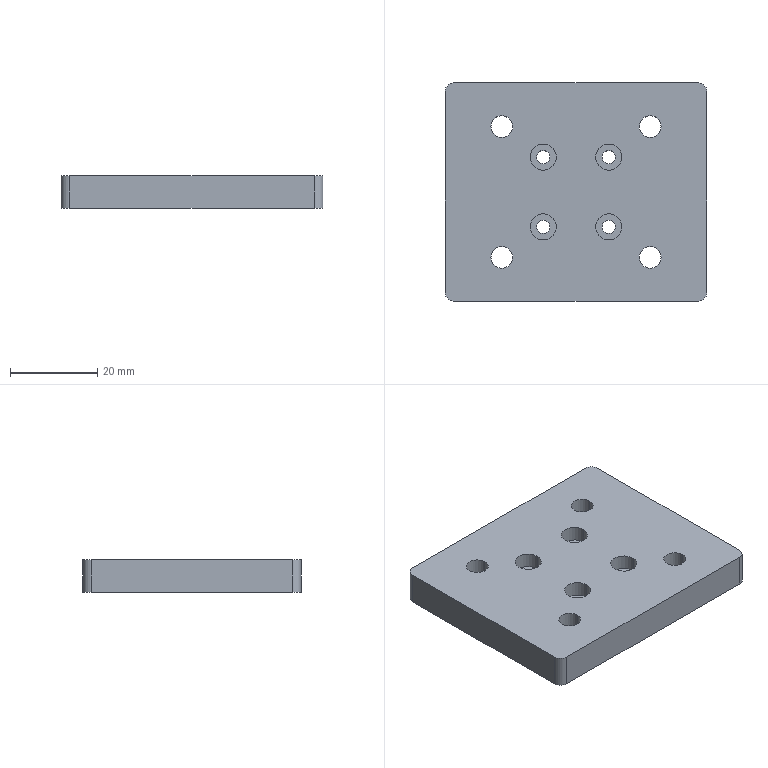Part | SolidWorks | features BaseBody 1 | 1 solid | 38 faces | box 60 x 50 x 7.5 mm | volume 21376 mm3 | cylinder 28 | plane 10 | commonest cylinder face diameters 3 x8 5 x8 6 x8 4 x4
STEP:
#1=CARTESIAN_POINT('',(19.5,-15.,7.5));
#2=VERTEX_POINT('',#1);
#3=CARTESIAN_POINT('',(14.5,-15.,7.5));
#4=VERTEX_POINT('',#3);
#5=CARTESIAN_POINT('',(17.,-15.,7.5));
#6=DIRECTION('',(0.,0.,-1.));
#7=DIRECTION('',(-1.,0.,0.));
#8=AXIS2_PLACEMENT_3D('',#5,#6,#7);
#9=CIRCLE('',#8,2.5);
#10=EDGE_CURVE('',#2,#4,#9,.T.);
#11=ORIENTED_EDGE('',*,*,#10,.F.);
#12=CARTESIAN_POINT('',(19.5,-15.,0.));
#13=VERTEX_POINT('',#12);
#14=CARTESIAN_POINT('',(19.5,-15.,7.5));
#15=DIRECTION('',(0.,0.,-1.));
#16=VECTOR('',#15,1000.);
#17=LINE('',#14,#16);
#18=EDGE_CURVE('',#2,#13,#17,.T.);
#19=ORIENTED_EDGE('',*,*,#18,.T.);
#20=CARTESIAN_POINT('',(14.5,-15.,0.));
#21=VERTEX_POINT('',#20);
#22=CARTESIAN_POINT('',(17.,-15.,0.));
#23=DIRECTION('',(0.,0.,-1.));
#24=DIRECTION('',(-1.,0.,0.));
#25=AXIS2_PLACEMENT_3D('',#22,#23,#24);
#26=CIRCLE('',#25,2.5);
#27=EDGE_CURVE('',#13,#21,#26,.T.);
#28=ORIENTED_EDGE('',*,*,#27,.T.);
#29=CARTESIAN_POINT('',(14.5,-15.,7.5));
#30=DIRECTION('',(0.,0.,-1.));
#31=VECTOR('',#30,1000.);
#32=LINE('',#29,#31);
#33=EDGE_CURVE('',#4,#21,#32,.T.);
#34=ORIENTED_EDGE('',*,*,#33,.F.);
#35=EDGE_LOOP('',(#11,#19,#28,#34));
#36=FACE_OUTER_BOUND('',#35,.T.);
#37=CARTESIAN_POINT('',(17.,-15.,7.5));
#38=DIRECTION('',(0.,0.,-1.));
#39=DIRECTION('',(-1.,0.,0.));
#40=AXIS2_PLACEMENT_3D('',#37,#38,#39);
#41=CYLINDRICAL_SURFACE('',#40,2.5);
#42=ADVANCED_FACE('',(#36),#41,.F.);
#43=CARTESIAN_POINT('',(19.5,15.,7.5));
#44=VERTEX_POINT('',#43);
#45=CARTESIAN_POINT('',(14.5,15.,7.5));
#46=VERTEX_POINT('',#45);
#47=CARTESIAN_POINT('',(17.,15.,7.5));
#48=DIRECTION('',(0.,0.,-1.));
#49=DIRECTION('',(-1.,0.,0.));
#50=AXIS2_PLACEMENT_3D('',#47,#48,#49);
#51=CIRCLE('',#50,2.5);
#52=EDGE_CURVE('',#44,#46,#51,.T.);
#53=ORIENTED_EDGE('',*,*,#52,.F.);
#54=CARTESIAN_POINT('',(19.5,15.,0.));
#55=VERTEX_POINT('',#54);
#56=CARTESIAN_POINT('',(19.5,15.,7.5));
#57=DIRECTION('',(0.,0.,-1.));
#58=VECTOR('',#57,1000.);
#59=LINE('',#56,#58);
#60=EDGE_CURVE('',#44,#55,#59,.T.);
#61=ORIENTED_EDGE('',*,*,#60,.T.);
#62=CARTESIAN_POINT('',(14.5,15.,0.));
#63=VERTEX_POINT('',#62);
#64=CARTESIAN_POINT('',(17.,15.,0.));
#65=DIRECTION('',(0.,0.,-1.));
#66=DIRECTION('',(-1.,0.,0.));
#67=AXIS2_PLACEMENT_3D('',#64,#65,#66);
#68=CIRCLE('',#67,2.5);
#69=EDGE_CURVE('',#55,#63,#68,.T.);
#70=ORIENTED_EDGE('',*,*,#69,.T.);
#71=CARTESIAN_POINT('',(14.5,15.,7.5));
#72=DIRECTION('',(0.,0.,-1.));
#73=VECTOR('',#72,1000.);
#74=LINE('',#71,#73);
#75=EDGE_CURVE('',#46,#63,#74,.T.);
#76=ORIENTED_EDGE('',*,*,#75,.F.);
#77=EDGE_LOOP('',(#53,#61,#70,#76));
#78=FACE_OUTER_BOUND('',#77,.T.);
#79=CARTESIAN_POINT('',(17.,15.,7.5));
#80=DIRECTION('',(0.,0.,-1.));
#81=DIRECTION('',(-1.,0.,0.));
#82=AXIS2_PLACEMENT_3D('',#79,#80,#81);
#83=CYLINDRICAL_SURFACE('',#82,2.5);
#84=ADVANCED_FACE('',(#78),#83,.F.);
#85=CARTESIAN_POINT('',(-6.,8.,4.));
#86=VERTEX_POINT('',#85);
#87=CARTESIAN_POINT('',(-9.,8.,4.));
#88=VERTEX_POINT('',#87);
#89=CARTESIAN_POINT('',(-7.5,8.,4.));
#90=DIRECTION('',(0.,0.,-1.));
#91=DIRECTION('',(-1.,0.,0.));
#92=AXIS2_PLACEMENT_3D('',#89,#90,#91);
#93=CIRCLE('',#92,1.5);
#94=EDGE_CURVE('',#86,#88,#93,.T.);
#95=ORIENTED_EDGE('',*,*,#94,.F.);
#96=CARTESIAN_POINT('',(-6.,8.,0.));
#97=VERTEX_POINT('',#96);
#98=CARTESIAN_POINT('',(-6.,8.,7.5));
#99=DIRECTION('',(0.,0.,-1.));
#100=VECTOR('',#99,1000.);
#101=LINE('',#98,#100);
#102=EDGE_CURVE('',#86,#97,#101,.T.);
#103=ORIENTED_EDGE('',*,*,#102,.T.);
#104=CARTESIAN_POINT('',(-9.,8.,0.));
#105=VERTEX_POINT('',#104);
#106=CARTESIAN_POINT('',(-7.5,8.,0.));
#107=DIRECTION('',(0.,0.,-1.));
#108=DIRECTION('',(-1.,0.,0.));
#109=AXIS2_PLACEMENT_3D('',#106,#107,#108);
#110=CIRCLE('',#109,1.5);
#111=EDGE_CURVE('',#97,#105,#110,.T.);
#112=ORIENTED_EDGE('',*,*,#111,.T.);
#113=CARTESIAN_POINT('',(-9.,8.,7.5));
#114=DIRECTION('',(0.,0.,-1.));
#115=VECTOR('',#114,1000.);
#116=LINE('',#113,#115);
#117=EDGE_CURVE('',#88,#105,#116,.T.);
#118=ORIENTED_EDGE('',*,*,#117,.F.);
#119=EDGE_LOOP('',(#95,#103,#112,#118));
#120=FACE_OUTER_BOUND('',#119,.T.);
#121=CARTESIAN_POINT('',(-7.5,8.,7.5));
#122=DIRECTION('',(0.,0.,-1.));
#123=DIRECTION('',(-1.,0.,0.));
#124=AXIS2_PLACEMENT_3D('',#121,#122,#123);
#125=CYLINDRICAL_SURFACE('',#124,1.5);
#126=ADVANCED_FACE('',(#120),#125,.F.);
#127=CARTESIAN_POINT('',(9.,8.,4.));
#128=VERTEX_POINT('',#127);
#129=CARTESIAN_POINT('',(6.,8.,4.));
#130=VERTEX_POINT('',#129);
#131=CARTESIAN_POINT('',(7.5,8.,4.));
#132=DIRECTION('',(0.,0.,-1.));
#133=DIRECTION('',(-1.,0.,0.));
#134=AXIS2_PLACEMENT_3D('',#131,#132,#133);
#135=CIRCLE('',#134,1.5);
#136=EDGE_CURVE('',#128,#130,#135,.T.);
#137=ORIENTED_EDGE('',*,*,#136,.F.);
#138=CARTESIAN_POINT('',(9.,8.,0.));
#139=VERTEX_POINT('',#138);
#140=CARTESIAN_POINT('',(9.,8.,7.5));
#141=DIRECTION('',(0.,0.,-1.));
#142=VECTOR('',#141,1000.);
#143=LINE('',#140,#142);
#144=EDGE_CURVE('',#128,#139,#143,.T.);
#145=ORIENTED_EDGE('',*,*,#144,.T.);
#146=CARTESIAN_POINT('',(6.,8.,0.));
#147=VERTEX_POINT('',#146);
#148=CARTESIAN_POINT('',(7.5,8.,0.));
#149=DIRECTION('',(0.,0.,-1.));
#150=DIRECTION('',(-1.,0.,0.));
#151=AXIS2_PLACEMENT_3D('',#148,#149,#150);
#152=CIRCLE('',#151,1.5);
#153=EDGE_CURVE('',#139,#147,#152,.T.);
#154=ORIENTED_EDGE('',*,*,#153,.T.);
#155=CARTESIAN_POINT('',(6.,8.,7.5));
#156=DIRECTION('',(0.,0.,-1.));
#157=VECTOR('',#156,1000.);
#158=LINE('',#155,#157);
#159=EDGE_CURVE('',#130,#147,#158,.T.);
#160=ORIENTED_EDGE('',*,*,#159,.F.);
#161=EDGE_LOOP('',(#137,#145,#154,#160));
#162=FACE_OUTER_BOUND('',#161,.T.);
#163=CARTESIAN_POINT('',(7.5,8.,7.5));
#164=DIRECTION('',(0.,0.,-1.));
#165=DIRECTION('',(-1.,0.,0.));
#166=AXIS2_PLACEMENT_3D('',#163,#164,#165);
#167=CYLINDRICAL_SURFACE('',#166,1.5);
#168=ADVANCED_FACE('',(#162),#167,.F.);
#169=CARTESIAN_POINT('',(9.,-8.,4.));
#170=VERTEX_POINT('',#169);
#171=CARTESIAN_POINT('',(6.,-8.,4.));
#172=VERTEX_POINT('',#171);
#173=CARTESIAN_POINT('',(7.5,-8.,4.));
#174=DIRECTION('',(0.,0.,-1.));
#175=DIRECTION('',(-1.,0.,0.));
#176=AXIS2_PLACEMENT_3D('',#173,#174,#175);
#177=CIRCLE('',#176,1.5);
#178=EDGE_CURVE('',#170,#172,#177,.T.);
#179=ORIENTED_EDGE('',*,*,#178,.F.);
#180=CARTESIAN_POINT('',(9.,-8.,0.));
#181=VERTEX_POINT('',#180);
#182=CARTESIAN_POINT('',(9.,-8.,7.5));
#183=DIRECTION('',(0.,0.,-1.));
#184=VECTOR('',#183,1000.);
#185=LINE('',#182,#184);
#186=EDGE_CURVE('',#170,#181,#185,.T.);
#187=ORIENTED_EDGE('',*,*,#186,.T.);
#188=CARTESIAN_POINT('',(6.,-8.,0.));
#189=VERTEX_POINT('',#188);
#190=CARTESIAN_POINT('',(7.5,-8.,0.));
#191=DIRECTION('',(0.,0.,-1.));
#192=DIRECTION('',(-1.,0.,0.));
#193=AXIS2_PLACEMENT_3D('',#190,#191,#192);
#194=CIRCLE('',#193,1.5);
#195=EDGE_CURVE('',#181,#189,#194,.T.);
#196=ORIENTED_EDGE('',*,*,#195,.T.);
#197=CARTESIAN_POINT('',(6.,-8.,7.5));
#198=DIRECTION('',(0.,0.,-1.));
#199=VECTOR('',#198,1000.);
#200=LINE('',#197,#199);
#201=EDGE_CURVE('',#172,#189,#200,.T.);
#202=ORIENTED_EDGE('',*,*,#201,.F.);
#203=EDGE_LOOP('',(#179,#187,#196,#202));
#204=FACE_OUTER_BOUND('',#203,.T.);
#205=CARTESIAN_POINT('',(7.5,-8.,7.5));
#206=DIRECTION('',(0.,0.,-1.));
#207=DIRECTION('',(-1.,0.,0.));
#208=AXIS2_PLACEMENT_3D('',#205,#206,#207);
#209=CYLINDRICAL_SURFACE('',#208,1.5);
#210=ADVANCED_FACE('',(#204),#209,.F.);
#211=CARTESIAN_POINT('',(-6.,-8.,4.));
#212=VERTEX_POINT('',#211);
#213=CARTESIAN_POINT('',(-9.,-8.,4.));
#214=VERTEX_POINT('',#213);
#215=CARTESIAN_POINT('',(-7.5,-8.,4.));
#216=DIRECTION('',(0.,0.,-1.));
#217=DIRECTION('',(-1.,0.,0.));
#218=AXIS2_PLACEMENT_3D('',#215,#216,#217);
#219=CIRCLE('',#218,1.5);
#220=EDGE_CURVE('',#212,#214,#219,.T.);
#221=ORIENTED_EDGE('',*,*,#220,.F.);
#222=CARTESIAN_POINT('',(-6.,-8.,0.));
#223=VERTEX_POINT('',#222);
#224=CARTESIAN_POINT('',(-6.,-8.,7.5));
#225=DIRECTION('',(0.,0.,-1.));
#226=VECTOR('',#225,1000.);
#227=LINE('',#224,#226);
#228=EDGE_CURVE('',#212,#223,#227,.T.);
#229=ORIENTED_EDGE('',*,*,#228,.T.);
#230=CARTESIAN_POINT('',(-9.,-8.,0.));
#231=VERTEX_POINT('',#230);
#232=CARTESIAN_POINT('',(-7.5,-8.,0.));
#233=DIRECTION('',(0.,0.,-1.));
#234=DIRECTION('',(-1.,0.,0.));
#235=AXIS2_PLACEMENT_3D('',#232,#233,#234);
#236=CIRCLE('',#235,1.5);
#237=EDGE_CURVE('',#223,#231,#236,.T.);
#238=ORIENTED_EDGE('',*,*,#237,.T.);
#239=CARTESIAN_POINT('',(-9.,-8.,7.5));
#240=DIRECTION('',(0.,0.,-1.));
#241=VECTOR('',#240,1000.);
#242=LINE('',#239,#241);
#243=EDGE_CURVE('',#214,#231,#242,.T.);
#244=ORIENTED_EDGE('',*,*,#243,.F.);
#245=EDGE_LOOP('',(#221,#229,#238,#244));
#246=FACE_OUTER_BOUND('',#245,.T.);
#247=CARTESIAN_POINT('',(-7.5,-8.,7.5));
#248=DIRECTION('',(0.,0.,-1.));
#249=DIRECTION('',(-1.,0.,0.));
#250=AXIS2_PLACEMENT_3D('',#247,#248,#249);
#251=CYLINDRICAL_SURFACE('',#250,1.5);
#252=ADVANCED_FACE('',(#246),#251,.F.);
#253=CARTESIAN_POINT('',(-14.5,15.,7.5));
#254=VERTEX_POINT('',#253);
#255=CARTESIAN_POINT('',(-19.5,15.,7.5));
#256=VERTEX_POINT('',#255);
#257=CARTESIAN_POINT('',(-17.,15.,7.5));
#258=DIRECTION('',(0.,0.,-1.));
#259=DIRECTION('',(-1.,0.,0.));
#260=AXIS2_PLACEMENT_3D('',#257,#258,#259);
#261=CIRCLE('',#260,2.5);
#262=EDGE_CURVE('',#254,#256,#261,.T.);
#263=ORIENTED_EDGE('',*,*,#262,.F.);
#264=CARTESIAN_POINT('',(-14.5,15.,0.));
#265=VERTEX_POINT('',#264);
#266=CARTESIAN_POINT('',(-14.5,15.,7.5));
#267=DIRECTION('',(0.,0.,-1.));
#268=VECTOR('',#267,1000.);
#269=LINE('',#266,#268);
#270=EDGE_CURVE('',#254,#265,#269,.T.);
#271=ORIENTED_EDGE('',*,*,#270,.T.);
#272=CARTESIAN_POINT('',(-19.5,15.,0.));
#273=VERTEX_POINT('',#272);
#274=CARTESIAN_POINT('',(-17.,15.,0.));
#275=DIRECTION('',(0.,0.,-1.));
#276=DIRECTION('',(-1.,0.,0.));
#277=AXIS2_PLACEMENT_3D('',#274,#275,#276);
#278=CIRCLE('',#277,2.5);
#279=EDGE_CURVE('',#265,#273,#278,.T.);
#280=ORIENTED_EDGE('',*,*,#279,.T.);
#281=CARTESIAN_POINT('',(-19.5,15.,7.5));
#282=DIRECTION('',(0.,0.,-1.));
#283=VECTOR('',#282,1000.);
#284=LINE('',#281,#283);
#285=EDGE_CURVE('',#256,#273,#284,.T.);
#286=ORIENTED_EDGE('',*,*,#285,.F.);
#287=EDGE_LOOP('',(#263,#271,#280,#286));
#288=FACE_OUTER_BOUND('',#287,.T.);
#289=CARTESIAN_POINT('',(-17.,15.,7.5));
#290=DIRECTION('',(0.,0.,-1.));
#291=DIRECTION('',(-1.,0.,0.));
#292=AXIS2_PLACEMENT_3D('',#289,#290,#291);
#293=CYLINDRICAL_SURFACE('',#292,2.5);
#294=ADVANCED_FACE('',(#288),#293,.F.);
#295=CARTESIAN_POINT('',(-14.5,-15.,7.5));
#296=VERTEX_POINT('',#295);
#297=CARTESIAN_POINT('',(-19.5,-15.,7.5));
#298=VERTEX_POINT('',#297);
#299=CARTESIAN_POINT('',(-17.,-15.,7.5));
#300=DIRECTION('',(0.,0.,-1.));
#301=DIRECTION('',(-1.,0.,0.));
#302=AXIS2_PLACEMENT_3D('',#299,#300,#301);
#303=CIRCLE('',#302,2.5);
#304=EDGE_CURVE('',#296,#298,#303,.T.);
#305=ORIENTED_EDGE('',*,*,#304,.F.);
#306=CARTESIAN_POINT('',(-14.5,-15.,0.));
#307=VERTEX_POINT('',#306);
#308=CARTESIAN_POINT('',(-14.5,-15.,7.5));
#309=DIRECTION('',(0.,0.,-1.));
#310=VECTOR('',#309,1000.);
#311=LINE('',#308,#310);
#312=EDGE_CURVE('',#296,#307,#311,.T.);
#313=ORIENTED_EDGE('',*,*,#312,.T.);
#314=CARTESIAN_POINT('',(-19.5,-15.,0.));
#315=VERTEX_POINT('',#314);
#316=CARTESIAN_POINT('',(-17.,-15.,0.));
#317=DIRECTION('',(0.,0.,-1.));
#318=DIRECTION('',(-1.,0.,0.));
#319=AXIS2_PLACEMENT_3D('',#316,#317,#318);
#320=CIRCLE('',#319,2.5);
#321=EDGE_CURVE('',#307,#315,#320,.T.);
#322=ORIENTED_EDGE('',*,*,#321,.T.);
#323=CARTESIAN_POINT('',(-19.5,-15.,7.5));
#324=DIRECTION('',(0.,0.,-1.));
#325=VECTOR('',#324,1000.);
#326=LINE('',#323,#325);
#327=EDGE_CURVE('',#298,#315,#326,.T.);
#328=ORIENTED_EDGE('',*,*,#327,.F.);
#329=EDGE_LOOP('',(#305,#313,#322,#328));
#330=FACE_OUTER_BOUND('',#329,.T.);
#331=CARTESIAN_POINT('',(-17.,-15.,7.5));
#332=DIRECTION('',(0.,0.,-1.));
#333=DIRECTION('',(-1.,0.,0.));
#334=AXIS2_PLACEMENT_3D('',#331,#332,#333);
#335=CYLINDRICAL_SURFACE('',#334,2.5);
#336=ADVANCED_FACE('',(#330),#335,.F.);
#337=CARTESIAN_POINT('',(-10.5,8.,4.));
#338=VERTEX_POINT('',#337);
#339=CARTESIAN_POINT('',(-4.5,8.,4.));
#340=VERTEX_POINT('',#339);
#341=CARTESIAN_POINT('',(-7.5,8.,4.));
#342=DIRECTION('',(0.,0.,1.));
#343=DIRECTION('',(1.,0.,0.));
#344=AXIS2_PLACEMENT_3D('',#341,#342,#343);
#345=CIRCLE('',#344,3.);
#346=EDGE_CURVE('',#338,#340,#345,.T.);
#347=ORIENTED_EDGE('',*,*,#346,.F.);
#348=CARTESIAN_POINT('',(-10.5,8.,7.5));
#349=VERTEX_POINT('',#348);
#350=CARTESIAN_POINT('',(-10.5,8.,4.));
#351=DIRECTION('',(0.,0.,1.));
#352=VECTOR('',#351,1000.);
#353=LINE('',#350,#352);
#354=EDGE_CURVE('',#338,#349,#353,.T.);
#355=ORIENTED_EDGE('',*,*,#354,.T.);
#356=CARTESIAN_POINT('',(-4.5,8.,7.5));
#357=VERTEX_POINT('',#356);
#358=CARTESIAN_POINT('',(-7.5,8.,7.5));
#359=DIRECTION('',(0.,0.,-1.));
#360=DIRECTION('',(1.,0.,0.));
#361=AXIS2_PLACEMENT_3D('',#358,#359,#360);
#362=CIRCLE('',#361,3.);
#363=EDGE_CURVE('',#357,#349,#362,.T.);
#364=ORIENTED_EDGE('',*,*,#363,.F.);
#365=CARTESIAN_POINT('',(-4.5,8.,4.));
#366=DIRECTION('',(0.,0.,1.));
#367=VECTOR('',#366,1000.);
#368=LINE('',#365,#367);
#369=EDGE_CURVE('',#340,#357,#368,.T.);
#370=ORIENTED_EDGE('',*,*,#369,.F.);
#371=EDGE_LOOP('',(#347,#355,#364,#370));
#372=FACE_OUTER_BOUND('',#371,.T.);
#373=CARTESIAN_POINT('',(-7.5,8.,4.));
#374=DIRECTION('',(0.,0.,1.));
#375=DIRECTION('',(1.,0.,0.));
#376=AXIS2_PLACEMENT_3D('',#373,#374,#375);
#377=CYLINDRICAL_SURFACE('',#376,3.);
#378=ADVANCED_FACE('',(#372),#377,.F.);
#379=CARTESIAN_POINT('',(4.5,-8.,4.));
#380=VERTEX_POINT('',#379);
#381=CARTESIAN_POINT('',(10.5,-8.,4.));
#382=VERTEX_POINT('',#381);
#383=CARTESIAN_POINT('',(7.5,-8.,4.));
#384=DIRECTION('',(0.,0.,1.));
#385=DIRECTION('',(1.,0.,0.));
#386=AXIS2_PLACEMENT_3D('',#383,#384,#385);
#387=CIRCLE('',#386,3.);
#388=EDGE_CURVE('',#380,#382,#387,.T.);
#389=ORIENTED_EDGE('',*,*,#388,.F.);
#390=CARTESIAN_POINT('',(4.5,-8.,7.5));
#391=VERTEX_POINT('',#390);
#392=CARTESIAN_POINT('',(4.5,-8.,4.));
#393=DIRECTION('',(0.,0.,1.));
#394=VECTOR('',#393,1000.);
#395=LINE('',#392,#394);
#396=EDGE_CURVE('',#380,#391,#395,.T.);
#397=ORIENTED_EDGE('',*,*,#396,.T.);
#398=CARTESIAN_POINT('',(10.5,-8.,7.5));
#399=VERTEX_POINT('',#398);
#400=CARTESIAN_POINT('',(7.5,-8.,7.5));
#401=DIRECTION('',(0.,0.,-1.));
#402=DIRECTION('',(1.,0.,0.));
#403=AXIS2_PLACEMENT_3D('',#400,#401,#402);
#404=CIRCLE('',#403,3.);
#405=EDGE_CURVE('',#399,#391,#404,.T.);
#406=ORIENTED_EDGE('',*,*,#405,.F.);
#407=CARTESIAN_POINT('',(10.5,-8.,4.));
#408=DIRECTION('',(0.,0.,1.));
#409=VECTOR('',#408,1000.);
#410=LINE('',#407,#409);
#411=EDGE_CURVE('',#382,#399,#410,.T.);
#412=ORIENTED_EDGE('',*,*,#411,.F.);
#413=EDGE_LOOP('',(#389,#397,#406,#412));
#414=FACE_OUTER_BOUND('',#413,.T.);
#415=CARTESIAN_POINT('',(7.5,-8.,4.));
#416=DIRECTION('',(0.,0.,1.));
#417=DIRECTION('',(1.,0.,0.));
#418=AXIS2_PLACEMENT_3D('',#415,#416,#417);
#419=CYLINDRICAL_SURFACE('',#418,3.);
#420=ADVANCED_FACE('',(#414),#419,.F.);
#421=CARTESIAN_POINT('',(-10.5,-8.,4.));
#422=VERTEX_POINT('',#421);
#423=CARTESIAN_POINT('',(-4.5,-8.,4.));
#424=VERTEX_POINT('',#423);
#425=CARTESIAN_POINT('',(-7.5,-8.,4.));
#426=DIRECTION('',(0.,0.,1.));
#427=DIRECTION('',(1.,0.,0.));
#428=AXIS2_PLACEMENT_3D('',#425,#426,#427);
#429=CIRCLE('',#428,3.);
#430=EDGE_CURVE('',#422,#424,#429,.T.);
#431=ORIENTED_EDGE('',*,*,#430,.F.);
#432=CARTESIAN_POINT('',(-10.5,-8.,7.5));
#433=VERTEX_POINT('',#432);
#434=CARTESIAN_POINT('',(-10.5,-8.,4.));
#435=DIRECTION('',(0.,0.,1.));
#436=VECTOR('',#435,1000.);
#437=LINE('',#434,#436);
#438=EDGE_CURVE('',#422,#433,#437,.T.);
#439=ORIENTED_EDGE('',*,*,#438,.T.);
#440=CARTESIAN_POINT('',(-4.5,-8.,7.5));
#441=VERTEX_POINT('',#440);
#442=CARTESIAN_POINT('',(-7.5,-8.,7.5));
#443=DIRECTION('',(0.,0.,-1.));
#444=DIRECTION('',(1.,0.,0.));
#445=AXIS2_PLACEMENT_3D('',#442,#443,#444);
#446=CIRCLE('',#445,3.);
#447=EDGE_CURVE('',#441,#433,#446,.T.);
#448=ORIENTED_EDGE('',*,*,#447,.F.);
#449=CARTESIAN_POINT('',(-4.5,-8.,4.));
#450=DIRECTION('',(0.,0.,1.));
#451=VECTOR('',#450,1000.);
#452=LINE('',#449,#451);
#453=EDGE_CURVE('',#424,#441,#452,.T.);
#454=ORIENTED_EDGE('',*,*,#453,.F.);
#455=EDGE_LOOP('',(#431,#439,#448,#454));
#456=FACE_OUTER_BOUND('',#455,.T.);
#457=CARTESIAN_POINT('',(-7.5,-8.,4.));
#458=DIRECTION('',(0.,0.,1.));
#459=DIRECTION('',(1.,0.,0.));
#460=AXIS2_PLACEMENT_3D('',#457,#458,#459);
#461=CYLINDRICAL_SURFACE('',#460,3.);
#462=ADVANCED_FACE('',(#456),#461,.F.);
#463=CARTESIAN_POINT('',(4.5,8.,4.));
#464=VERTEX_POINT('',#463);
#465=CARTESIAN_POINT('',(10.5,8.,4.));
#466=VERTEX_POINT('',#465);
#467=CARTESIAN_POINT('',(7.5,8.,4.));
#468=DIRECTION('',(0.,0.,1.));
#469=DIRECTION('',(1.,0.,0.));
#470=AXIS2_PLACEMENT_3D('',#467,#468,#469);
#471=CIRCLE('',#470,3.);
#472=EDGE_CURVE('',#464,#466,#471,.T.);
#473=ORIENTED_EDGE('',*,*,#472,.F.);
#474=CARTESIAN_POINT('',(4.5,8.,7.5));
#475=VERTEX_POINT('',#474);
#476=CARTESIAN_POINT('',(4.5,8.,4.));
#477=DIRECTION('',(0.,0.,1.));
#478=VECTOR('',#477,1000.);
#479=LINE('',#476,#478);
#480=EDGE_CURVE('',#464,#475,#479,.T.);
#481=ORIENTED_EDGE('',*,*,#480,.T.);
#482=CARTESIAN_POINT('',(10.5,8.,7.5));
#483=VERTEX_POINT('',#482);
#484=CARTESIAN_POINT('',(7.5,8.,7.5));
#485=DIRECTION('',(0.,0.,-1.));
#486=DIRECTION('',(1.,0.,0.));
#487=AXIS2_PLACEMENT_3D('',#484,#485,#486);
#488=CIRCLE('',#487,3.);
#489=EDGE_CURVE('',#483,#475,#488,.T.);
#490=ORIENTED_EDGE('',*,*,#489,.F.);
#491=CARTESIAN_POINT('',(10.5,8.,4.));
#492=DIRECTION('',(0.,0.,1.));
#493=VECTOR('',#492,1000.);
#494=LINE('',#491,#493);
#495=EDGE_CURVE('',#466,#483,#494,.T.);
#496=ORIENTED_EDGE('',*,*,#495,.F.);
#497=EDGE_LOOP('',(#473,#481,#490,#496));
#498=FACE_OUTER_BOUND('',#497,.T.);
#499=CARTESIAN_POINT('',(7.5,8.,4.));
#500=DIRECTION('',(0.,0.,1.));
#501=DIRECTION('',(1.,0.,0.));
#502=AXIS2_PLACEMENT_3D('',#499,#500,#501);
#503=CYLINDRICAL_SURFACE('',#502,3.);
#504=ADVANCED_FACE('',(#498),#503,.F.);
#505=CARTESIAN_POINT('',(17.,-15.,0.));
#506=DIRECTION('',(0.,0.,-1.));
#507=DIRECTION('',(-1.,0.,0.));
#508=AXIS2_PLACEMENT_3D('',#505,#506,#507);
#509=CIRCLE('',#508,2.5);
#510=EDGE_CURVE('',#21,#13,#509,.T.);
#511=ORIENTED_EDGE('',*,*,#510,.F.);
#512=ORIENTED_EDGE('',*,*,#27,.F.);
#513=EDGE_LOOP('',(#511,#512));
#514=FACE_BOUND('',#513,.T.);
#515=CARTESIAN_POINT('',(17.,15.,0.));
#516=DIRECTION('',(0.,0.,-1.));
#517=DIRECTION('',(-1.,0.,0.));
#518=AXIS2_PLACEMENT_3D('',#515,#516,#517);
#519=CIRCLE('',#518,2.5);
#520=EDGE_CURVE('',#63,#55,#519,.T.);
#521=ORIENTED_EDGE('',*,*,#520,.F.);
#522=ORIENTED_EDGE('',*,*,#69,.F.);
#523=EDGE_LOOP('',(#521,#522));
#524=FACE_BOUND('',#523,.T.);
#525=CARTESIAN_POINT('',(-7.5,8.,0.));
#526=DIRECTION('',(0.,0.,-1.));
#527=DIRECTION('',(-1.,0.,0.));
#528=AXIS2_PLACEMENT_3D('',#525,#526,#527);
#529=CIRCLE('',#528,1.5);
#530=EDGE_CURVE('',#105,#97,#529,.T.);
#531=ORIENTED_EDGE('',*,*,#530,.F.);
#532=ORIENTED_EDGE('',*,*,#111,.F.);
#533=EDGE_LOOP('',(#531,#532));
#534=FACE_BOUND('',#533,.T.);
#535=CARTESIAN_POINT('',(7.5,8.,0.));
#536=DIRECTION('',(0.,0.,-1.));
#537=DIRECTION('',(-1.,0.,0.));
#538=AXIS2_PLACEMENT_3D('',#535,#536,#537);
#539=CIRCLE('',#538,1.5);
#540=EDGE_CURVE('',#147,#139,#539,.T.);
#541=ORIENTED_EDGE('',*,*,#540,.F.);
#542=ORIENTED_EDGE('',*,*,#153,.F.);
#543=EDGE_LOOP('',(#541,#542));
#544=FACE_BOUND('',#543,.T.);
#545=CARTESIAN_POINT('',(7.5,-8.,0.));
#546=DIRECTION('',(0.,0.,-1.));
#547=DIRECTION('',(-1.,0.,0.));
#548=AXIS2_PLACEMENT_3D('',#545,#546,#547);
#549=CIRCLE('',#548,1.5);
#550=EDGE_CURVE('',#189,#181,#549,.T.);
#551=ORIENTED_EDGE('',*,*,#550,.F.);
#552=ORIENTED_EDGE('',*,*,#195,.F.);
#553=EDGE_LOOP('',(#551,#552));
#554=FACE_BOUND('',#553,.T.);
#555=CARTESIAN_POINT('',(-7.5,-8.,0.));
#556=DIRECTION('',(0.,0.,-1.));
#557=DIRECTION('',(-1.,0.,0.));
#558=AXIS2_PLACEMENT_3D('',#555,#556,#557);
#559=CIRCLE('',#558,1.5);
#560=EDGE_CURVE('',#231,#223,#559,.T.);
#561=ORIENTED_EDGE('',*,*,#560,.F.);
#562=ORIENTED_EDGE('',*,*,#237,.F.);
#563=EDGE_LOOP('',(#561,#562));
#564=FACE_BOUND('',#563,.T.);
#565=CARTESIAN_POINT('',(-30.,-23.,0.));
#566=VERTEX_POINT('',#565);
#567=CARTESIAN_POINT('',(-28.,-25.,0.));
#568=VERTEX_POINT('',#567);
#569=CARTESIAN_POINT('',(-28.,-23.,0.));
#570=DIRECTION('',(0.,0.,1.));
#571=DIRECTION('',(-1.,0.,0.));
#572=AXIS2_PLACEMENT_3D('',#569,#570,#571);
#573=CIRCLE('',#572,2.);
#574=EDGE_CURVE('',#566,#568,#573,.T.);
#575=ORIENTED_EDGE('',*,*,#574,.F.);
#576=CARTESIAN_POINT('',(-30.,23.,0.));
#577=VERTEX_POINT('',#576);
#578=CARTESIAN_POINT('',(-30.,0.,0.));
#579=DIRECTION('',(0.,-1.,0.));
#580=VECTOR('',#579,1000.);
#581=LINE('',#578,#580);
#582=EDGE_CURVE('',#577,#566,#581,.T.);
#583=ORIENTED_EDGE('',*,*,#582,.F.);
#584=CARTESIAN_POINT('',(-28.,25.,0.));
#585=VERTEX_POINT('',#584);
#586=CARTESIAN_POINT('',(-28.,23.,0.));
#587=DIRECTION('',(0.,0.,1.));
#588=DIRECTION('',(-1.,0.,0.));
#589=AXIS2_PLACEMENT_3D('',#586,#587,#588);
#590=CIRCLE('',#589,2.);
#591=EDGE_CURVE('',#585,#577,#590,.T.);
#592=ORIENTED_EDGE('',*,*,#591,.F.);
#593=CARTESIAN_POINT('',(28.,25.,0.));
#594=VERTEX_POINT('',#593);
#595=CARTESIAN_POINT('',(0.,25.,0.));
#596=DIRECTION('',(-1.,0.,0.));
#597=VECTOR('',#596,1000.);
#598=LINE('',#595,#597);
#599=EDGE_CURVE('',#594,#585,#598,.T.);
#600=ORIENTED_EDGE('',*,*,#599,.F.);
#601=CARTESIAN_POINT('',(30.,23.,0.));
#602=VERTEX_POINT('',#601);
#603=CARTESIAN_POINT('',(28.,23.,0.));
#604=DIRECTION('',(0.,0.,1.));
#605=DIRECTION('',(1.,0.,0.));
#606=AXIS2_PLACEMENT_3D('',#603,#604,#605);
#607=CIRCLE('',#606,2.);
#608=EDGE_CURVE('',#602,#594,#607,.T.);
#609=ORIENTED_EDGE('',*,*,#608,.F.);
#610=CARTESIAN_POINT('',(30.,-23.,0.));
#611=VERTEX_POINT('',#610);
#612=CARTESIAN_POINT('',(30.,0.,0.));
#613=DIRECTION('',(0.,1.,0.));
#614=VECTOR('',#613,1000.);
#615=LINE('',#612,#614);
#616=EDGE_CURVE('',#611,#602,#615,.T.);
#617=ORIENTED_EDGE('',*,*,#616,.F.);
#618=CARTESIAN_POINT('',(28.,-25.,0.));
#619=VERTEX_POINT('',#618);
#620=CARTESIAN_POINT('',(28.,-23.,0.));
#621=DIRECTION('',(0.,0.,1.));
#622=DIRECTION('',(1.,0.,0.));
#623=AXIS2_PLACEMENT_3D('',#620,#621,#622);
#624=CIRCLE('',#623,2.);
#625=EDGE_CURVE('',#619,#611,#624,.T.);
#626=ORIENTED_EDGE('',*,*,#625,.F.);
#627=CARTESIAN_POINT('',(0.,-25.,0.));
#628=DIRECTION('',(1.,0.,0.));
#629=VECTOR('',#628,1000.);
#630=LINE('',#627,#629);
#631=EDGE_CURVE('',#568,#619,#630,.T.);
#632=ORIENTED_EDGE('',*,*,#631,.F.);
#633=EDGE_LOOP('',(#575,#583,#592,#600,#609,#617,#626,#632));
#634=FACE_OUTER_BOUND('',#633,.T.);
#635=CARTESIAN_POINT('',(-17.,15.,0.));
#636=DIRECTION('',(0.,0.,-1.));
#637=DIRECTION('',(-1.,0.,0.));
#638=AXIS2_PLACEMENT_3D('',#635,#636,#637);
#639=CIRCLE('',#638,2.5);
#640=EDGE_CURVE('',#273,#265,#639,.T.);
#641=ORIENTED_EDGE('',*,*,#640,.F.);
#642=ORIENTED_EDGE('',*,*,#279,.F.);
#643=EDGE_LOOP('',(#641,#642));
#644=FACE_BOUND('',#643,.T.);
#645=CARTESIAN_POINT('',(-17.,-15.,0.));
#646=DIRECTION('',(0.,0.,-1.));
#647=DIRECTION('',(-1.,0.,0.));
#648=AXIS2_PLACEMENT_3D('',#645,#646,#647);
#649=CIRCLE('',#648,2.5);
#650=EDGE_CURVE('',#315,#307,#649,.T.);
#651=ORIENTED_EDGE('',*,*,#650,.F.);
#652=ORIENTED_EDGE('',*,*,#321,.F.);
#653=EDGE_LOOP('',(#651,#652));
#654=FACE_BOUND('',#653,.T.);
#655=CARTESIAN_POINT('',(0.,0.,0.));
#656=DIRECTION('',(0.,0.,1.));
#657=DIRECTION('',(1.,0.,0.));
#658=AXIS2_PLACEMENT_3D('',#655,#656,#657);
#659=PLANE('',#658);
#660=ADVANCED_FACE('',(#514,#524,#534,#544,#554,#564,#634,#644,#654),#659,.F.);
#661=ORIENTED_EDGE('',*,*,#18,.F.);
#662=CARTESIAN_POINT('',(17.,-15.,7.5));
#663=DIRECTION('',(0.,0.,-1.));
#664=DIRECTION('',(-1.,0.,0.));
#665=AXIS2_PLACEMENT_3D('',#662,#663,#664);
#666=CIRCLE('',#665,2.5);
#667=EDGE_CURVE('',#4,#2,#666,.T.);
#668=ORIENTED_EDGE('',*,*,#667,.F.);
#669=ORIENTED_EDGE('',*,*,#33,.T.);
#670=ORIENTED_EDGE('',*,*,#510,.T.);
#671=EDGE_LOOP('',(#661,#668,#669,#670));
#672=FACE_OUTER_BOUND('',#671,.T.);
#673=CARTESIAN_POINT('',(17.,-15.,7.5));
#674=DIRECTION('',(0.,0.,-1.));
#675=DIRECTION('',(-1.,0.,0.));
#676=AXIS2_PLACEMENT_3D('',#673,#674,#675);
#677=CYLINDRICAL_SURFACE('',#676,2.5);
#678=ADVANCED_FACE('',(#672),#677,.F.);
#679=ORIENTED_EDGE('',*,*,#60,.F.);
#680=CARTESIAN_POINT('',(17.,15.,7.5));
#681=DIRECTION('',(0.,0.,-1.));
#682=DIRECTION('',(-1.,0.,0.));
#683=AXIS2_PLACEMENT_3D('',#680,#681,#682);
#684=CIRCLE('',#683,2.5);
#685=EDGE_CURVE('',#46,#44,#684,.T.);
#686=ORIENTED_EDGE('',*,*,#685,.F.);
#687=ORIENTED_EDGE('',*,*,#75,.T.);
#688=ORIENTED_EDGE('',*,*,#520,.T.);
#689=EDGE_LOOP('',(#679,#686,#687,#688));
#690=FACE_OUTER_BOUND('',#689,.T.);
#691=CARTESIAN_POINT('',(17.,15.,7.5));
#692=DIRECTION('',(0.,0.,-1.));
#693=DIRECTION('',(-1.,0.,0.));
#694=AXIS2_PLACEMENT_3D('',#691,#692,#693);
#695=CYLINDRICAL_SURFACE('',#694,2.5);
#696=ADVANCED_FACE('',(#690),#695,.F.);
#697=ORIENTED_EDGE('',*,*,#102,.F.);
#698=CARTESIAN_POINT('',(-7.5,8.,4.));
#699=DIRECTION('',(0.,0.,-1.));
#700=DIRECTION('',(-1.,0.,0.));
#701=AXIS2_PLACEMENT_3D('',#698,#699,#700);
#702=CIRCLE('',#701,1.5);
#703=EDGE_CURVE('',#88,#86,#702,.T.);
#704=ORIENTED_EDGE('',*,*,#703,.F.);
#705=ORIENTED_EDGE('',*,*,#117,.T.);
#706=ORIENTED_EDGE('',*,*,#530,.T.);
#707=EDGE_LOOP('',(#697,#704,#705,#706));
#708=FACE_OUTER_BOUND('',#707,.T.);
#709=CARTESIAN_POINT('',(-7.5,8.,7.5));
#710=DIRECTION('',(0.,0.,-1.));
#711=DIRECTION('',(-1.,0.,0.));
#712=AXIS2_PLACEMENT_3D('',#709,#710,#711);
#713=CYLINDRICAL_SURFACE('',#712,1.5);
#714=ADVANCED_FACE('',(#708),#713,.F.);
#715=ORIENTED_EDGE('',*,*,#144,.F.);
#716=CARTESIAN_POINT('',(7.5,8.,4.));
#717=DIRECTION('',(0.,0.,-1.));
#718=DIRECTION('',(-1.,0.,0.));
#719=AXIS2_PLACEMENT_3D('',#716,#717,#718);
#720=CIRCLE('',#719,1.5);
#721=EDGE_CURVE('',#130,#128,#720,.T.);
#722=ORIENTED_EDGE('',*,*,#721,.F.);
#723=ORIENTED_EDGE('',*,*,#159,.T.);
#724=ORIENTED_EDGE('',*,*,#540,.T.);
#725=EDGE_LOOP('',(#715,#722,#723,#724));
#726=FACE_OUTER_BOUND('',#725,.T.);
#727=CARTESIAN_POINT('',(7.5,8.,7.5));
#728=DIRECTION('',(0.,0.,-1.));
#729=DIRECTION('',(-1.,0.,0.));
#730=AXIS2_PLACEMENT_3D('',#727,#728,#729);
#731=CYLINDRICAL_SURFACE('',#730,1.5);
#732=ADVANCED_FACE('',(#726),#731,.F.);
#733=ORIENTED_EDGE('',*,*,#186,.F.);
#734=CARTESIAN_POINT('',(7.5,-8.,4.));
#735=DIRECTION('',(0.,0.,-1.));
#736=DIRECTION('',(-1.,0.,0.));
#737=AXIS2_PLACEMENT_3D('',#734,#735,#736);
#738=CIRCLE('',#737,1.5);
#739=EDGE_CURVE('',#172,#170,#738,.T.);
#740=ORIENTED_EDGE('',*,*,#739,.F.);
#741=ORIENTED_EDGE('',*,*,#201,.T.);
#742=ORIENTED_EDGE('',*,*,#550,.T.);
#743=EDGE_LOOP('',(#733,#740,#741,#742));
#744=FACE_OUTER_BOUND('',#743,.T.);
#745=CARTESIAN_POINT('',(7.5,-8.,7.5));
#746=DIRECTION('',(0.,0.,-1.));
#747=DIRECTION('',(-1.,0.,0.));
#748=AXIS2_PLACEMENT_3D('',#745,#746,#747);
#749=CYLINDRICAL_SURFACE('',#748,1.5);
#750=ADVANCED_FACE('',(#744),#749,.F.);
#751=ORIENTED_EDGE('',*,*,#228,.F.);
#752=CARTESIAN_POINT('',(-7.5,-8.,4.));
#753=DIRECTION('',(0.,0.,-1.));
#754=DIRECTION('',(-1.,0.,0.));
#755=AXIS2_PLACEMENT_3D('',#752,#753,#754);
#756=CIRCLE('',#755,1.5);
#757=EDGE_CURVE('',#214,#212,#756,.T.);
#758=ORIENTED_EDGE('',*,*,#757,.F.);
#759=ORIENTED_EDGE('',*,*,#243,.T.);
#760=ORIENTED_EDGE('',*,*,#560,.T.);
#761=EDGE_LOOP('',(#751,#758,#759,#760));
#762=FACE_OUTER_BOUND('',#761,.T.);
#763=CARTESIAN_POINT('',(-7.5,-8.,7.5));
#764=DIRECTION('',(0.,0.,-1.));
#765=DIRECTION('',(-1.,0.,0.));
#766=AXIS2_PLACEMENT_3D('',#763,#764,#765);
#767=CYLINDRICAL_SURFACE('',#766,1.5);
#768=ADVANCED_FACE('',(#762),#767,.F.);
#769=CARTESIAN_POINT('',(-28.,-25.,7.5));
#770=VERTEX_POINT('',#769);
#771=CARTESIAN_POINT('',(-28.,-25.,7.5));
#772=DIRECTION('',(0.,0.,1.));
#773=VECTOR('',#772,1000.);
#774=LINE('',#771,#773);
#775=EDGE_CURVE('',#568,#770,#774,.T.);
#776=ORIENTED_EDGE('',*,*,#775,.F.);
#777=ORIENTED_EDGE('',*,*,#631,.T.);
#778=CARTESIAN_POINT('',(28.,-25.,7.5));
#779=VERTEX_POINT('',#778);
#780=CARTESIAN_POINT('',(28.,-25.,7.5));
#781=DIRECTION('',(0.,0.,-1.));
#782=VECTOR('',#781,1000.);
#783=LINE('',#780,#782);
#784=EDGE_CURVE('',#779,#619,#783,.T.);
#785=ORIENTED_EDGE('',*,*,#784,.F.);
#786=CARTESIAN_POINT('',(0.,-25.,7.5));
#787=DIRECTION('',(1.,0.,0.));
#788=VECTOR('',#787,1000.);
#789=LINE('',#786,#788);
#790=EDGE_CURVE('',#770,#779,#789,.T.);
#791=ORIENTED_EDGE('',*,*,#790,.F.);
#792=EDGE_LOOP('',(#776,#777,#785,#791));
#793=FACE_OUTER_BOUND('',#792,.T.);
#794=CARTESIAN_POINT('',(0.,-25.,7.5));
#795=DIRECTION('',(0.,1.,0.));
#796=DIRECTION('',(-1.,0.,0.));
#797=AXIS2_PLACEMENT_3D('',#794,#795,#796);
#798=PLANE('',#797);
#799=ADVANCED_FACE('',(#793),#798,.F.);
#800=ORIENTED_EDGE('',*,*,#574,.T.);
#801=ORIENTED_EDGE('',*,*,#775,.T.);
#802=CARTESIAN_POINT('',(-30.,-23.,7.5));
#803=VERTEX_POINT('',#802);
#804=CARTESIAN_POINT('',(-28.,-23.,7.5));
#805=DIRECTION('',(0.,0.,-1.));
#806=DIRECTION('',(-1.,0.,0.));
#807=AXIS2_PLACEMENT_3D('',#804,#805,#806);
#808=CIRCLE('',#807,2.);
#809=EDGE_CURVE('',#770,#803,#808,.T.);
#810=ORIENTED_EDGE('',*,*,#809,.T.);
#811=CARTESIAN_POINT('',(-30.,-23.,7.5));
#812=DIRECTION('',(0.,0.,-1.));
#813=VECTOR('',#812,1000.);
#814=LINE('',#811,#813);
#815=EDGE_CURVE('',#803,#566,#814,.T.);
#816=ORIENTED_EDGE('',*,*,#815,.T.);
#817=EDGE_LOOP('',(#800,#801,#810,#816));
#818=FACE_OUTER_BOUND('',#817,.T.);
#819=CARTESIAN_POINT('',(-28.,-23.,7.5));
#820=DIRECTION('',(0.,0.,-1.));
#821=DIRECTION('',(-1.,0.,0.));
#822=AXIS2_PLACEMENT_3D('',#819,#820,#821);
#823=CYLINDRICAL_SURFACE('',#822,2.);
#824=ADVANCED_FACE('',(#818),#823,.T.);
#825=ORIENTED_EDGE('',*,*,#815,.F.);
#826=CARTESIAN_POINT('',(-30.,23.,7.5));
#827=VERTEX_POINT('',#826);
#828=CARTESIAN_POINT('',(-30.,0.,7.5));
#829=DIRECTION('',(0.,-1.,0.));
#830=VECTOR('',#829,1000.);
#831=LINE('',#828,#830);
#832=EDGE_CURVE('',#827,#803,#831,.T.);
#833=ORIENTED_EDGE('',*,*,#832,.F.);
#834=CARTESIAN_POINT('',(-30.,23.,7.5));
#835=DIRECTION('',(0.,0.,1.));
#836=VECTOR('',#835,1000.);
#837=LINE('',#834,#836);
#838=EDGE_CURVE('',#577,#827,#837,.T.);
#839=ORIENTED_EDGE('',*,*,#838,.F.);
#840=ORIENTED_EDGE('',*,*,#582,.T.);
#841=EDGE_LOOP('',(#825,#833,#839,#840));
#842=FACE_OUTER_BOUND('',#841,.T.);
#843=CARTESIAN_POINT('',(-30.,0.,7.5));
#844=DIRECTION('',(1.,0.,0.));
#845=DIRECTION('',(0.,0.,-1.));
#846=AXIS2_PLACEMENT_3D('',#843,#844,#845);
#847=PLANE('',#846);
#848=ADVANCED_FACE('',(#842),#847,.F.);
#849=ORIENTED_EDGE('',*,*,#591,.T.);
#850=ORIENTED_EDGE('',*,*,#838,.T.);
#851=CARTESIAN_POINT('',(-28.,25.,7.5));
#852=VERTEX_POINT('',#851);
#853=CARTESIAN_POINT('',(-28.,23.,7.5));
#854=DIRECTION('',(0.,0.,-1.));
#855=DIRECTION('',(-1.,0.,0.));
#856=AXIS2_PLACEMENT_3D('',#853,#854,#855);
#857=CIRCLE('',#856,2.);
#858=EDGE_CURVE('',#827,#852,#857,.T.);
#859=ORIENTED_EDGE('',*,*,#858,.T.);
#860=CARTESIAN_POINT('',(-28.,25.,7.5));
#861=DIRECTION('',(0.,0.,-1.));
#862=VECTOR('',#861,1000.);
#863=LINE('',#860,#862);
#864=EDGE_CURVE('',#852,#585,#863,.T.);
#865=ORIENTED_EDGE('',*,*,#864,.T.);
#866=EDGE_LOOP('',(#849,#850,#859,#865));
#867=FACE_OUTER_BOUND('',#866,.T.);
#868=CARTESIAN_POINT('',(-28.,23.,7.5));
#869=DIRECTION('',(0.,0.,-1.));
#870=DIRECTION('',(-1.,0.,0.));
#871=AXIS2_PLACEMENT_3D('',#868,#869,#870);
#872=CYLINDRICAL_SURFACE('',#871,2.);
#873=ADVANCED_FACE('',(#867),#872,.T.);
#874=CARTESIAN_POINT('',(28.,25.,7.5));
#875=VERTEX_POINT('',#874);
#876=CARTESIAN_POINT('',(28.,25.,7.5));
#877=DIRECTION('',(0.,0.,1.));
#878=VECTOR('',#877,1000.);
#879=LINE('',#876,#878);
#880=EDGE_CURVE('',#594,#875,#879,.T.);
#881=ORIENTED_EDGE('',*,*,#880,.F.);
#882=ORIENTED_EDGE('',*,*,#599,.T.);
#883=ORIENTED_EDGE('',*,*,#864,.F.);
#884=CARTESIAN_POINT('',(0.,25.,7.5));
#885=DIRECTION('',(-1.,0.,0.));
#886=VECTOR('',#885,1000.);
#887=LINE('',#884,#886);
#888=EDGE_CURVE('',#875,#852,#887,.T.);
#889=ORIENTED_EDGE('',*,*,#888,.F.);
#890=EDGE_LOOP('',(#881,#882,#883,#889));
#891=FACE_OUTER_BOUND('',#890,.T.);
#892=CARTESIAN_POINT('',(0.,25.,7.5));
#893=DIRECTION('',(0.,-1.,0.));
#894=DIRECTION('',(0.,0.,-1.));
#895=AXIS2_PLACEMENT_3D('',#892,#893,#894);
#896=PLANE('',#895);
#897=ADVANCED_FACE('',(#891),#896,.F.);
#898=ORIENTED_EDGE('',*,*,#608,.T.);
#899=ORIENTED_EDGE('',*,*,#880,.T.);
#900=CARTESIAN_POINT('',(30.,23.,7.5));
#901=VERTEX_POINT('',#900);
#902=CARTESIAN_POINT('',(28.,23.,7.5));
#903=DIRECTION('',(0.,0.,-1.));
#904=DIRECTION('',(1.,0.,0.));
#905=AXIS2_PLACEMENT_3D('',#902,#903,#904);
#906=CIRCLE('',#905,2.);
#907=EDGE_CURVE('',#875,#901,#906,.T.);
#908=ORIENTED_EDGE('',*,*,#907,.T.);
#909=CARTESIAN_POINT('',(30.,23.,7.5));
#910=DIRECTION('',(0.,0.,-1.));
#911=VECTOR('',#910,1000.);
#912=LINE('',#909,#911);
#913=EDGE_CURVE('',#901,#602,#912,.T.);
#914=ORIENTED_EDGE('',*,*,#913,.T.);
#915=EDGE_LOOP('',(#898,#899,#908,#914));
#916=FACE_OUTER_BOUND('',#915,.T.);
#917=CARTESIAN_POINT('',(28.,23.,7.5));
#918=DIRECTION('',(0.,0.,1.));
#919=DIRECTION('',(1.,0.,0.));
#920=AXIS2_PLACEMENT_3D('',#917,#918,#919);
#921=CYLINDRICAL_SURFACE('',#920,2.);
#922=ADVANCED_FACE('',(#916),#921,.T.);
#923=ORIENTED_EDGE('',*,*,#616,.T.);
#924=ORIENTED_EDGE('',*,*,#913,.F.);
#925=CARTESIAN_POINT('',(30.,-23.,7.5));
#926=VERTEX_POINT('',#925);
#927=CARTESIAN_POINT('',(30.,0.,7.5));
#928=DIRECTION('',(0.,-1.,0.));
#929=VECTOR('',#928,1000.);
#930=LINE('',#927,#929);
#931=EDGE_CURVE('',#901,#926,#930,.T.);
#932=ORIENTED_EDGE('',*,*,#931,.T.);
#933=CARTESIAN_POINT('',(30.,-23.,7.5));
#934=DIRECTION('',(0.,0.,-1.));
#935=VECTOR('',#934,1000.);
#936=LINE('',#933,#935);
#937=EDGE_CURVE('',#926,#611,#936,.T.);
#938=ORIENTED_EDGE('',*,*,#937,.T.);
#939=EDGE_LOOP('',(#923,#924,#932,#938));
#940=FACE_OUTER_BOUND('',#939,.T.);
#941=CARTESIAN_POINT('',(30.,0.,7.5));
#942=DIRECTION('',(1.,0.,0.));
#943=DIRECTION('',(0.,1.,0.));
#944=AXIS2_PLACEMENT_3D('',#941,#942,#943);
#945=PLANE('',#944);
#946=ADVANCED_FACE('',(#940),#945,.T.);
#947=ORIENTED_EDGE('',*,*,#625,.T.);
#948=ORIENTED_EDGE('',*,*,#937,.F.);
#949=CARTESIAN_POINT('',(28.,-23.,7.5));
#950=DIRECTION('',(0.,0.,-1.));
#951=DIRECTION('',(1.,0.,0.));
#952=AXIS2_PLACEMENT_3D('',#949,#950,#951);
#953=CIRCLE('',#952,2.);
#954=EDGE_CURVE('',#926,#779,#953,.T.);
#955=ORIENTED_EDGE('',*,*,#954,.T.);
#956=ORIENTED_EDGE('',*,*,#784,.T.);
#957=EDGE_LOOP('',(#947,#948,#955,#956));
#958=FACE_OUTER_BOUND('',#957,.T.);
#959=CARTESIAN_POINT('',(28.,-23.,7.5));
#960=DIRECTION('',(0.,0.,1.));
#961=DIRECTION('',(1.,0.,0.));
#962=AXIS2_PLACEMENT_3D('',#959,#960,#961);
#963=CYLINDRICAL_SURFACE('',#962,2.);
#964=ADVANCED_FACE('',(#958),#963,.T.);
#965=ORIENTED_EDGE('',*,*,#270,.F.);
#966=CARTESIAN_POINT('',(-17.,15.,7.5));
#967=DIRECTION('',(0.,0.,-1.));
#968=DIRECTION('',(-1.,0.,0.));
#969=AXIS2_PLACEMENT_3D('',#966,#967,#968);
#970=CIRCLE('',#969,2.5);
#971=EDGE_CURVE('',#256,#254,#970,.T.);
#972=ORIENTED_EDGE('',*,*,#971,.F.);
#973=ORIENTED_EDGE('',*,*,#285,.T.);
#974=ORIENTED_EDGE('',*,*,#640,.T.);
#975=EDGE_LOOP('',(#965,#972,#973,#974));
#976=FACE_OUTER_BOUND('',#975,.T.);
#977=CARTESIAN_POINT('',(-17.,15.,7.5));
#978=DIRECTION('',(0.,0.,-1.));
#979=DIRECTION('',(-1.,0.,0.));
#980=AXIS2_PLACEMENT_3D('',#977,#978,#979);
#981=CYLINDRICAL_SURFACE('',#980,2.5);
#982=ADVANCED_FACE('',(#976),#981,.F.);
#983=ORIENTED_EDGE('',*,*,#312,.F.);
#984=CARTESIAN_POINT('',(-17.,-15.,7.5));
#985=DIRECTION('',(0.,0.,-1.));
#986=DIRECTION('',(-1.,0.,0.));
#987=AXIS2_PLACEMENT_3D('',#984,#985,#986);
#988=CIRCLE('',#987,2.5);
#989=EDGE_CURVE('',#298,#296,#988,.T.);
#990=ORIENTED_EDGE('',*,*,#989,.F.);
#991=ORIENTED_EDGE('',*,*,#327,.T.);
#992=ORIENTED_EDGE('',*,*,#650,.T.);
#993=EDGE_LOOP('',(#983,#990,#991,#992));
#994=FACE_OUTER_BOUND('',#993,.T.);
#995=CARTESIAN_POINT('',(-17.,-15.,7.5));
#996=DIRECTION('',(0.,0.,-1.));
#997=DIRECTION('',(-1.,0.,0.));
#998=AXIS2_PLACEMENT_3D('',#995,#996,#997);
#999=CYLINDRICAL_SURFACE('',#998,2.5);
#1000=ADVANCED_FACE('',(#994),#999,.F.);
#1001=ORIENTED_EDGE('',*,*,#667,.T.);
#1002=ORIENTED_EDGE('',*,*,#10,.T.);
#1003=EDGE_LOOP('',(#1001,#1002));
#1004=FACE_BOUND('',#1003,.T.);
#1005=ORIENTED_EDGE('',*,*,#685,.T.);
#1006=ORIENTED_EDGE('',*,*,#52,.T.);
#1007=EDGE_LOOP('',(#1005,#1006));
#1008=FACE_BOUND('',#1007,.T.);
#1009=ORIENTED_EDGE('',*,*,#888,.T.);
#1010=ORIENTED_EDGE('',*,*,#858,.F.);
#1011=ORIENTED_EDGE('',*,*,#832,.T.);
#1012=ORIENTED_EDGE('',*,*,#809,.F.);
#1013=ORIENTED_EDGE('',*,*,#790,.T.);
#1014=ORIENTED_EDGE('',*,*,#954,.F.);
#1015=ORIENTED_EDGE('',*,*,#931,.F.);
#1016=ORIENTED_EDGE('',*,*,#907,.F.);
#1017=EDGE_LOOP('',(#1009,#1010,#1011,#1012,#1013,#1014,#1015,#1016));
#1018=FACE_OUTER_BOUND('',#1017,.T.);
#1019=ORIENTED_EDGE('',*,*,#971,.T.);
#1020=ORIENTED_EDGE('',*,*,#262,.T.);
#1021=EDGE_LOOP('',(#1019,#1020));
#1022=FACE_BOUND('',#1021,.T.);
#1023=ORIENTED_EDGE('',*,*,#989,.T.);
#1024=ORIENTED_EDGE('',*,*,#304,.T.);
#1025=EDGE_LOOP('',(#1023,#1024));
#1026=FACE_BOUND('',#1025,.T.);
#1027=ORIENTED_EDGE('',*,*,#363,.T.);
#1028=CARTESIAN_POINT('',(-7.5,8.,7.5));
#1029=DIRECTION('',(0.,0.,-1.));
#1030=DIRECTION('',(1.,0.,0.));
#1031=AXIS2_PLACEMENT_3D('',#1028,#1029,#1030);
#1032=CIRCLE('',#1031,3.);
#1033=EDGE_CURVE('',#349,#357,#1032,.T.);
#1034=ORIENTED_EDGE('',*,*,#1033,.T.);
#1035=EDGE_LOOP('',(#1027,#1034));
#1036=FACE_BOUND('',#1035,.T.);
#1037=ORIENTED_EDGE('',*,*,#405,.T.);
#1038=CARTESIAN_POINT('',(7.5,-8.,7.5));
#1039=DIRECTION('',(0.,0.,-1.));
#1040=DIRECTION('',(1.,0.,0.));
#1041=AXIS2_PLACEMENT_3D('',#1038,#1039,#1040);
#1042=CIRCLE('',#1041,3.);
#1043=EDGE_CURVE('',#391,#399,#1042,.T.);
#1044=ORIENTED_EDGE('',*,*,#1043,.T.);
#1045=EDGE_LOOP('',(#1037,#1044));
#1046=FACE_BOUND('',#1045,.T.);
#1047=ORIENTED_EDGE('',*,*,#447,.T.);
#1048=CARTESIAN_POINT('',(-7.5,-8.,7.5));
#1049=DIRECTION('',(0.,0.,-1.));
#1050=DIRECTION('',(1.,0.,0.));
#1051=AXIS2_PLACEMENT_3D('',#1048,#1049,#1050);
#1052=CIRCLE('',#1051,3.);
#1053=EDGE_CURVE('',#433,#441,#1052,.T.);
#1054=ORIENTED_EDGE('',*,*,#1053,.T.);
#1055=EDGE_LOOP('',(#1047,#1054));
#1056=FACE_BOUND('',#1055,.T.);
#1057=ORIENTED_EDGE('',*,*,#489,.T.);
#1058=CARTESIAN_POINT('',(7.5,8.,7.5));
#1059=DIRECTION('',(0.,0.,-1.));
#1060=DIRECTION('',(1.,0.,0.));
#1061=AXIS2_PLACEMENT_3D('',#1058,#1059,#1060);
#1062=CIRCLE('',#1061,3.);
#1063=EDGE_CURVE('',#475,#483,#1062,.T.);
#1064=ORIENTED_EDGE('',*,*,#1063,.T.);
#1065=EDGE_LOOP('',(#1057,#1064));
#1066=FACE_BOUND('',#1065,.T.);
#1067=CARTESIAN_POINT('',(0.,0.,7.5));
#1068=DIRECTION('',(0.,0.,1.));
#1069=DIRECTION('',(1.,0.,0.));
#1070=AXIS2_PLACEMENT_3D('',#1067,#1068,#1069);
#1071=PLANE('',#1070);
#1072=ADVANCED_FACE('',(#1004,#1008,#1018,#1022,#1026,#1036,#1046,#1056,#1066),#1071,.T.);
#1073=CARTESIAN_POINT('',(-7.5,8.,4.));
#1074=DIRECTION('',(0.,0.,1.));
#1075=DIRECTION('',(1.,0.,0.));
#1076=AXIS2_PLACEMENT_3D('',#1073,#1074,#1075);
#1077=CIRCLE('',#1076,3.);
#1078=EDGE_CURVE('',#340,#338,#1077,.T.);
#1079=ORIENTED_EDGE('',*,*,#1078,.T.);
#1080=ORIENTED_EDGE('',*,*,#346,.T.);
#1081=EDGE_LOOP('',(#1079,#1080));
#1082=FACE_OUTER_BOUND('',#1081,.T.);
#1083=ORIENTED_EDGE('',*,*,#703,.T.);
#1084=ORIENTED_EDGE('',*,*,#94,.T.);
#1085=EDGE_LOOP('',(#1083,#1084));
#1086=FACE_BOUND('',#1085,.T.);
#1087=CARTESIAN_POINT('',(-7.5,8.,4.));
#1088=DIRECTION('',(0.,0.,1.));
#1089=DIRECTION('',(1.,0.,0.));
#1090=AXIS2_PLACEMENT_3D('',#1087,#1088,#1089);
#1091=PLANE('',#1090);
#1092=ADVANCED_FACE('',(#1082,#1086),#1091,.T.);
#1093=CARTESIAN_POINT('',(7.5,8.,4.));
#1094=DIRECTION('',(0.,0.,1.));
#1095=DIRECTION('',(1.,0.,0.));
#1096=AXIS2_PLACEMENT_3D('',#1093,#1094,#1095);
#1097=CIRCLE('',#1096,3.);
#1098=EDGE_CURVE('',#466,#464,#1097,.T.);
#1099=ORIENTED_EDGE('',*,*,#1098,.T.);
#1100=ORIENTED_EDGE('',*,*,#472,.T.);
#1101=EDGE_LOOP('',(#1099,#1100));
#1102=FACE_OUTER_BOUND('',#1101,.T.);
#1103=ORIENTED_EDGE('',*,*,#721,.T.);
#1104=ORIENTED_EDGE('',*,*,#136,.T.);
#1105=EDGE_LOOP('',(#1103,#1104));
#1106=FACE_BOUND('',#1105,.T.);
#1107=CARTESIAN_POINT('',(7.5,8.,4.));
#1108=DIRECTION('',(0.,0.,1.));
#1109=DIRECTION('',(1.,0.,0.));
#1110=AXIS2_PLACEMENT_3D('',#1107,#1108,#1109);
#1111=PLANE('',#1110);
#1112=ADVANCED_FACE('',(#1102,#1106),#1111,.T.);
#1113=CARTESIAN_POINT('',(7.5,-8.,4.));
#1114=DIRECTION('',(0.,0.,1.));
#1115=DIRECTION('',(1.,0.,0.));
#1116=AXIS2_PLACEMENT_3D('',#1113,#1114,#1115);
#1117=CIRCLE('',#1116,3.);
#1118=EDGE_CURVE('',#382,#380,#1117,.T.);
#1119=ORIENTED_EDGE('',*,*,#1118,.T.);
#1120=ORIENTED_EDGE('',*,*,#388,.T.);
#1121=EDGE_LOOP('',(#1119,#1120));
#1122=FACE_OUTER_BOUND('',#1121,.T.);
#1123=ORIENTED_EDGE('',*,*,#739,.T.);
#1124=ORIENTED_EDGE('',*,*,#178,.T.);
#1125=EDGE_LOOP('',(#1123,#1124));
#1126=FACE_BOUND('',#1125,.T.);
#1127=CARTESIAN_POINT('',(7.5,-8.,4.));
#1128=DIRECTION('',(0.,0.,1.));
#1129=DIRECTION('',(1.,0.,0.));
#1130=AXIS2_PLACEMENT_3D('',#1127,#1128,#1129);
#1131=PLANE('',#1130);
#1132=ADVANCED_FACE('',(#1122,#1126),#1131,.T.);
#1133=CARTESIAN_POINT('',(-7.5,-8.,4.));
#1134=DIRECTION('',(0.,0.,1.));
#1135=DIRECTION('',(1.,0.,0.));
#1136=AXIS2_PLACEMENT_3D('',#1133,#1134,#1135);
#1137=CIRCLE('',#1136,3.);
#1138=EDGE_CURVE('',#424,#422,#1137,.T.);
#1139=ORIENTED_EDGE('',*,*,#1138,.T.);
#1140=ORIENTED_EDGE('',*,*,#430,.T.);
#1141=EDGE_LOOP('',(#1139,#1140));
#1142=FACE_OUTER_BOUND('',#1141,.T.);
#1143=ORIENTED_EDGE('',*,*,#757,.T.);
#1144=ORIENTED_EDGE('',*,*,#220,.T.);
#1145=EDGE_LOOP('',(#1143,#1144));
#1146=FACE_BOUND('',#1145,.T.);
#1147=CARTESIAN_POINT('',(-7.5,-8.,4.));
#1148=DIRECTION('',(0.,0.,1.));
#1149=DIRECTION('',(1.,0.,0.));
#1150=AXIS2_PLACEMENT_3D('',#1147,#1148,#1149);
#1151=PLANE('',#1150);
#1152=ADVANCED_FACE('',(#1142,#1146),#1151,.T.);
#1153=ORIENTED_EDGE('',*,*,#354,.F.);
#1154=ORIENTED_EDGE('',*,*,#1078,.F.);
#1155=ORIENTED_EDGE('',*,*,#369,.T.);
#1156=ORIENTED_EDGE('',*,*,#1033,.F.);
#1157=EDGE_LOOP('',(#1153,#1154,#1155,#1156));
#1158=FACE_OUTER_BOUND('',#1157,.T.);
#1159=CARTESIAN_POINT('',(-7.5,8.,4.));
#1160=DIRECTION('',(0.,0.,1.));
#1161=DIRECTION('',(1.,0.,0.));
#1162=AXIS2_PLACEMENT_3D('',#1159,#1160,#1161);
#1163=CYLINDRICAL_SURFACE('',#1162,3.);
#1164=ADVANCED_FACE('',(#1158),#1163,.F.);
#1165=ORIENTED_EDGE('',*,*,#396,.F.);
#1166=ORIENTED_EDGE('',*,*,#1118,.F.);
#1167=ORIENTED_EDGE('',*,*,#411,.T.);
#1168=ORIENTED_EDGE('',*,*,#1043,.F.);
#1169=EDGE_LOOP('',(#1165,#1166,#1167,#1168));
#1170=FACE_OUTER_BOUND('',#1169,.T.);
#1171=CARTESIAN_POINT('',(7.5,-8.,4.));
#1172=DIRECTION('',(0.,0.,1.));
#1173=DIRECTION('',(1.,0.,0.));
#1174=AXIS2_PLACEMENT_3D('',#1171,#1172,#1173);
#1175=CYLINDRICAL_SURFACE('',#1174,3.);
#1176=ADVANCED_FACE('',(#1170),#1175,.F.);
#1177=ORIENTED_EDGE('',*,*,#438,.F.);
#1178=ORIENTED_EDGE('',*,*,#1138,.F.);
#1179=ORIENTED_EDGE('',*,*,#453,.T.);
#1180=ORIENTED_EDGE('',*,*,#1053,.F.);
#1181=EDGE_LOOP('',(#1177,#1178,#1179,#1180));
#1182=FACE_OUTER_BOUND('',#1181,.T.);
#1183=CARTESIAN_POINT('',(-7.5,-8.,4.));
#1184=DIRECTION('',(0.,0.,1.));
#1185=DIRECTION('',(1.,0.,0.));
#1186=AXIS2_PLACEMENT_3D('',#1183,#1184,#1185);
#1187=CYLINDRICAL_SURFACE('',#1186,3.);
#1188=ADVANCED_FACE('',(#1182),#1187,.F.);
#1189=ORIENTED_EDGE('',*,*,#480,.F.);
#1190=ORIENTED_EDGE('',*,*,#1098,.F.);
#1191=ORIENTED_EDGE('',*,*,#495,.T.);
#1192=ORIENTED_EDGE('',*,*,#1063,.F.);
#1193=EDGE_LOOP('',(#1189,#1190,#1191,#1192));
#1194=FACE_OUTER_BOUND('',#1193,.T.);
#1195=CARTESIAN_POINT('',(7.5,8.,4.));
#1196=DIRECTION('',(0.,0.,1.));
#1197=DIRECTION('',(1.,0.,0.));
#1198=AXIS2_PLACEMENT_3D('',#1195,#1196,#1197);
#1199=CYLINDRICAL_SURFACE('',#1198,3.);
#1200=ADVANCED_FACE('',(#1194),#1199,.F.);
#1201=CLOSED_SHELL('',(#42,#84,#126,#168,#210,#252,#294,#336,#378,#420,#462,#504,#660,#678,#696,#714,#732,#750,#768,#799,#824,#848,#873,#897,#922,#946,#964,#982,#1000,#1072,#1092,#1112,#1132,#1152,#1164,#1176,#1188,#1200));
#1202=MANIFOLD_SOLID_BREP('',#1201);
#1203=CARTESIAN_POINT('',(0.,0.,0.));
#1204=DIRECTION('',(0.,0.,1.));
#1205=DIRECTION('',(1.,0.,0.));
#1206=AXIS2_PLACEMENT_3D('',#1203,#1204,#1205);
#1207=(LENGTH_UNIT()NAMED_UNIT(*)SI_UNIT(.MILLI.,.METRE.));
#1208=UNCERTAINTY_MEASURE_WITH_UNIT(LENGTH_MEASURE(0.00001),#1207,'','');
#1209=(NAMED_UNIT(*)PLANE_ANGLE_UNIT()SI_UNIT($,.RADIAN.));
#1210=(NAMED_UNIT(*)SI_UNIT($,.STERADIAN.)SOLID_ANGLE_UNIT());
#1211=(GEOMETRIC_REPRESENTATION_CONTEXT(3)GLOBAL_UNCERTAINTY_ASSIGNED_CONTEXT((#1208))GLOBAL_UNIT_ASSIGNED_CONTEXT((#1207,#1209,#1210))REPRESENTATION_CONTEXT('',''));
#1212=ADVANCED_BREP_SHAPE_REPRESENTATION('',(#1202,#1206),#1211);